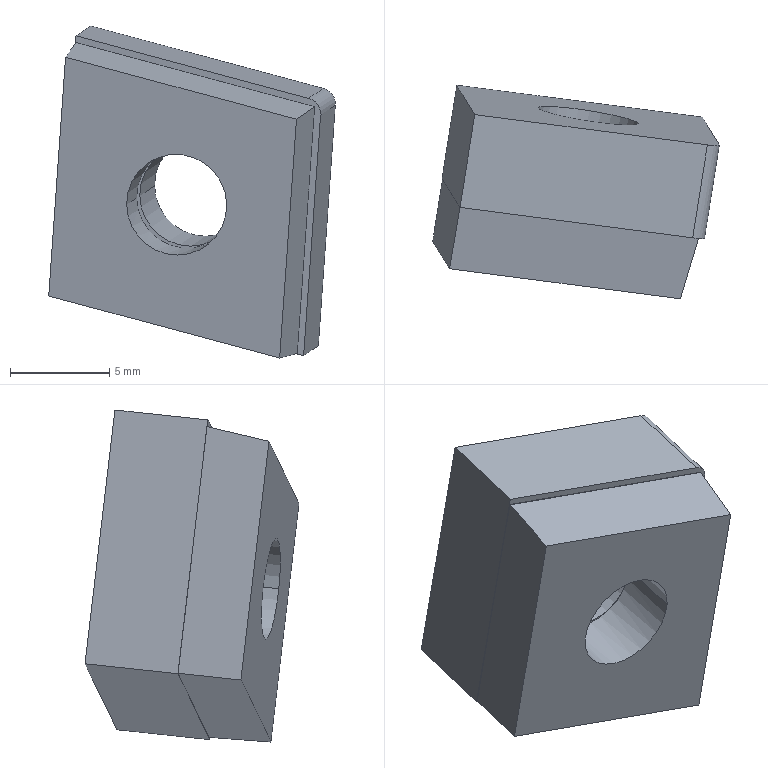Part | 2 solids | 19 faces | volume 1099 mm3 | plane 14 | cylinder 5 | commonest cylinder face diameters 5.1 x4 1.6 x1